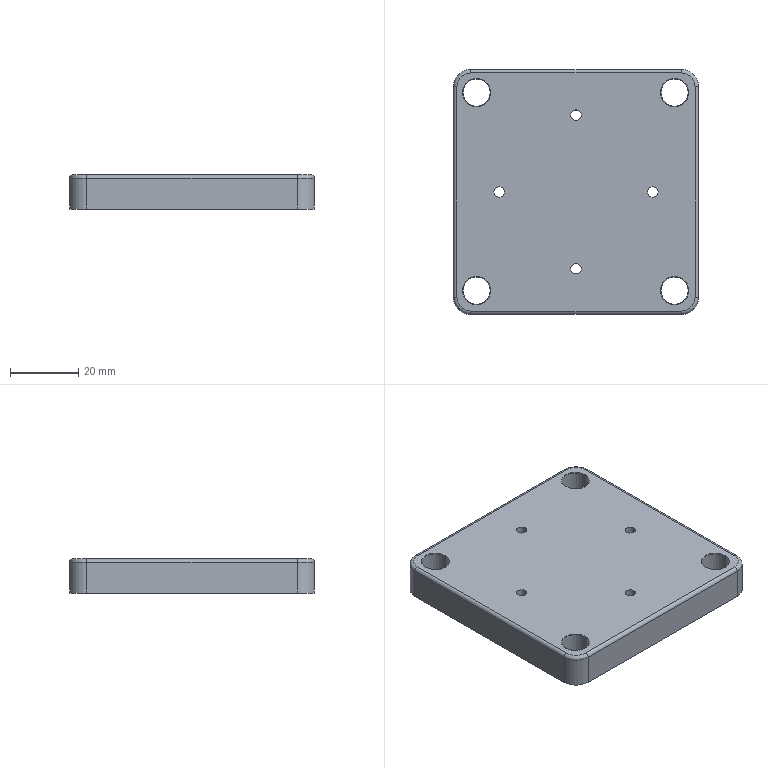Part | SolidWorks | features Fillet 3, Extrusion 1, ICE 1 | 1 solid | 42 faces | box 71.75 x 71.75 x 10 mm | volume 48903 mm3 | cylinder 24 | torus 12 | plane 6 | commonest cylinder face diameters 3.05 x8 8 x8 2 x4 10 x4
STEP:
#1=CARTESIAN_POINT('',(-1.525,22.5,0.));
#2=VERTEX_POINT('',#1);
#3=CARTESIAN_POINT('',(1.525,22.5,0.));
#4=VERTEX_POINT('',#3);
#5=CARTESIAN_POINT('',(0.,22.5,0.));
#6=DIRECTION('',(0.,0.,1.));
#7=DIRECTION('',(1.,0.,0.));
#8=AXIS2_PLACEMENT_3D('',#5,#6,#7);
#9=CIRCLE('',#8,1.525);
#10=EDGE_CURVE('',#2,#4,#9,.T.);
#11=ORIENTED_EDGE('',*,*,#10,.F.);
#12=CARTESIAN_POINT('',(-1.525,22.5,10.));
#13=VERTEX_POINT('',#12);
#14=CARTESIAN_POINT('',(-1.525,22.5,0.));
#15=DIRECTION('',(0.,0.,1.));
#16=VECTOR('',#15,1000.);
#17=LINE('',#14,#16);
#18=EDGE_CURVE('',#2,#13,#17,.T.);
#19=ORIENTED_EDGE('',*,*,#18,.T.);
#20=CARTESIAN_POINT('',(1.525,22.5,10.));
#21=VERTEX_POINT('',#20);
#22=CARTESIAN_POINT('',(0.,22.5,10.));
#23=DIRECTION('',(0.,0.,1.));
#24=DIRECTION('',(1.,0.,0.));
#25=AXIS2_PLACEMENT_3D('',#22,#23,#24);
#26=CIRCLE('',#25,1.525);
#27=EDGE_CURVE('',#13,#21,#26,.T.);
#28=ORIENTED_EDGE('',*,*,#27,.T.);
#29=CARTESIAN_POINT('',(1.525,22.5,0.));
#30=DIRECTION('',(0.,0.,1.));
#31=VECTOR('',#30,1000.);
#32=LINE('',#29,#31);
#33=EDGE_CURVE('',#4,#21,#32,.T.);
#34=ORIENTED_EDGE('',*,*,#33,.F.);
#35=EDGE_LOOP('',(#11,#19,#28,#34));
#36=FACE_OUTER_BOUND('',#35,.T.);
#37=CARTESIAN_POINT('',(0.,22.5,0.));
#38=DIRECTION('',(0.,0.,1.));
#39=DIRECTION('',(1.,0.,0.));
#40=AXIS2_PLACEMENT_3D('',#37,#38,#39);
#41=CYLINDRICAL_SURFACE('',#40,1.525);
#42=ADVANCED_FACE('',(#36),#41,.F.);
#43=CARTESIAN_POINT('',(20.975,0.,0.));
#44=VERTEX_POINT('',#43);
#45=CARTESIAN_POINT('',(24.025,0.,0.));
#46=VERTEX_POINT('',#45);
#47=CARTESIAN_POINT('',(22.5,0.,0.));
#48=DIRECTION('',(0.,0.,1.));
#49=DIRECTION('',(1.,0.,0.));
#50=AXIS2_PLACEMENT_3D('',#47,#48,#49);
#51=CIRCLE('',#50,1.525);
#52=EDGE_CURVE('',#44,#46,#51,.T.);
#53=ORIENTED_EDGE('',*,*,#52,.F.);
#54=CARTESIAN_POINT('',(20.975,0.,10.));
#55=VERTEX_POINT('',#54);
#56=CARTESIAN_POINT('',(20.975,0.,0.));
#57=DIRECTION('',(0.,0.,1.));
#58=VECTOR('',#57,1000.);
#59=LINE('',#56,#58);
#60=EDGE_CURVE('',#44,#55,#59,.T.);
#61=ORIENTED_EDGE('',*,*,#60,.T.);
#62=CARTESIAN_POINT('',(24.025,0.,10.));
#63=VERTEX_POINT('',#62);
#64=CARTESIAN_POINT('',(22.5,0.,10.));
#65=DIRECTION('',(0.,0.,1.));
#66=DIRECTION('',(1.,0.,0.));
#67=AXIS2_PLACEMENT_3D('',#64,#65,#66);
#68=CIRCLE('',#67,1.525);
#69=EDGE_CURVE('',#55,#63,#68,.T.);
#70=ORIENTED_EDGE('',*,*,#69,.T.);
#71=CARTESIAN_POINT('',(24.025,0.,0.));
#72=DIRECTION('',(0.,0.,1.));
#73=VECTOR('',#72,1000.);
#74=LINE('',#71,#73);
#75=EDGE_CURVE('',#46,#63,#74,.T.);
#76=ORIENTED_EDGE('',*,*,#75,.F.);
#77=EDGE_LOOP('',(#53,#61,#70,#76));
#78=FACE_OUTER_BOUND('',#77,.T.);
#79=CARTESIAN_POINT('',(22.5,0.,0.));
#80=DIRECTION('',(0.,0.,1.));
#81=DIRECTION('',(1.,0.,0.));
#82=AXIS2_PLACEMENT_3D('',#79,#80,#81);
#83=CYLINDRICAL_SURFACE('',#82,1.525);
#84=ADVANCED_FACE('',(#78),#83,.F.);
#85=CARTESIAN_POINT('',(-1.525,-22.5,0.));
#86=VERTEX_POINT('',#85);
#87=CARTESIAN_POINT('',(1.525,-22.5,0.));
#88=VERTEX_POINT('',#87);
#89=CARTESIAN_POINT('',(0.,-22.5,0.));
#90=DIRECTION('',(0.,0.,1.));
#91=DIRECTION('',(1.,0.,0.));
#92=AXIS2_PLACEMENT_3D('',#89,#90,#91);
#93=CIRCLE('',#92,1.525);
#94=EDGE_CURVE('',#86,#88,#93,.T.);
#95=ORIENTED_EDGE('',*,*,#94,.F.);
#96=CARTESIAN_POINT('',(-1.525,-22.5,10.));
#97=VERTEX_POINT('',#96);
#98=CARTESIAN_POINT('',(-1.525,-22.5,0.));
#99=DIRECTION('',(0.,0.,1.));
#100=VECTOR('',#99,1000.);
#101=LINE('',#98,#100);
#102=EDGE_CURVE('',#86,#97,#101,.T.);
#103=ORIENTED_EDGE('',*,*,#102,.T.);
#104=CARTESIAN_POINT('',(1.525,-22.5,10.));
#105=VERTEX_POINT('',#104);
#106=CARTESIAN_POINT('',(0.,-22.5,10.));
#107=DIRECTION('',(0.,0.,1.));
#108=DIRECTION('',(1.,0.,0.));
#109=AXIS2_PLACEMENT_3D('',#106,#107,#108);
#110=CIRCLE('',#109,1.525);
#111=EDGE_CURVE('',#97,#105,#110,.T.);
#112=ORIENTED_EDGE('',*,*,#111,.T.);
#113=CARTESIAN_POINT('',(1.525,-22.5,0.));
#114=DIRECTION('',(0.,0.,1.));
#115=VECTOR('',#114,1000.);
#116=LINE('',#113,#115);
#117=EDGE_CURVE('',#88,#105,#116,.T.);
#118=ORIENTED_EDGE('',*,*,#117,.F.);
#119=EDGE_LOOP('',(#95,#103,#112,#118));
#120=FACE_OUTER_BOUND('',#119,.T.);
#121=CARTESIAN_POINT('',(0.,-22.5,0.));
#122=DIRECTION('',(0.,0.,1.));
#123=DIRECTION('',(1.,0.,0.));
#124=AXIS2_PLACEMENT_3D('',#121,#122,#123);
#125=CYLINDRICAL_SURFACE('',#124,1.525);
#126=ADVANCED_FACE('',(#120),#125,.F.);
#127=CARTESIAN_POINT('',(-24.025,0.,0.));
#128=VERTEX_POINT('',#127);
#129=CARTESIAN_POINT('',(-20.975,0.,0.));
#130=VERTEX_POINT('',#129);
#131=CARTESIAN_POINT('',(-22.5,0.,0.));
#132=DIRECTION('',(0.,0.,1.));
#133=DIRECTION('',(1.,0.,0.));
#134=AXIS2_PLACEMENT_3D('',#131,#132,#133);
#135=CIRCLE('',#134,1.525);
#136=EDGE_CURVE('',#128,#130,#135,.T.);
#137=ORIENTED_EDGE('',*,*,#136,.F.);
#138=CARTESIAN_POINT('',(-24.025,0.,10.));
#139=VERTEX_POINT('',#138);
#140=CARTESIAN_POINT('',(-24.025,0.,0.));
#141=DIRECTION('',(0.,0.,1.));
#142=VECTOR('',#141,1000.);
#143=LINE('',#140,#142);
#144=EDGE_CURVE('',#128,#139,#143,.T.);
#145=ORIENTED_EDGE('',*,*,#144,.T.);
#146=CARTESIAN_POINT('',(-20.975,0.,10.));
#147=VERTEX_POINT('',#146);
#148=CARTESIAN_POINT('',(-22.5,0.,10.));
#149=DIRECTION('',(0.,0.,1.));
#150=DIRECTION('',(1.,0.,0.));
#151=AXIS2_PLACEMENT_3D('',#148,#149,#150);
#152=CIRCLE('',#151,1.525);
#153=EDGE_CURVE('',#139,#147,#152,.T.);
#154=ORIENTED_EDGE('',*,*,#153,.T.);
#155=CARTESIAN_POINT('',(-20.975,0.,0.));
#156=DIRECTION('',(0.,0.,1.));
#157=VECTOR('',#156,1000.);
#158=LINE('',#155,#157);
#159=EDGE_CURVE('',#130,#147,#158,.T.);
#160=ORIENTED_EDGE('',*,*,#159,.F.);
#161=EDGE_LOOP('',(#137,#145,#154,#160));
#162=FACE_OUTER_BOUND('',#161,.T.);
#163=CARTESIAN_POINT('',(-22.5,0.,0.));
#164=DIRECTION('',(0.,0.,1.));
#165=DIRECTION('',(1.,0.,0.));
#166=AXIS2_PLACEMENT_3D('',#163,#164,#165);
#167=CYLINDRICAL_SURFACE('',#166,1.525);
#168=ADVANCED_FACE('',(#162),#167,.F.);
#169=CARTESIAN_POINT('',(24.725,29.125,10.));
#170=VERTEX_POINT('',#169);
#171=CARTESIAN_POINT('',(33.025,29.125,10.));
#172=VERTEX_POINT('',#171);
#173=CARTESIAN_POINT('',(28.875,29.125,10.));
#174=DIRECTION('',(0.,0.,-1.));
#175=DIRECTION('',(1.,0.,0.));
#176=AXIS2_PLACEMENT_3D('',#173,#174,#175);
#177=CIRCLE('',#176,4.15);
#178=EDGE_CURVE('',#170,#172,#177,.T.);
#179=ORIENTED_EDGE('',*,*,#178,.F.);
#180=CARTESIAN_POINT('',(24.875,29.125,9.85));
#181=VERTEX_POINT('',#180);
#182=CARTESIAN_POINT('',(24.725,29.125,9.85));
#183=DIRECTION('',(0.,1.,0.));
#184=DIRECTION('',(-1.,0.,0.));
#185=AXIS2_PLACEMENT_3D('',#182,#183,#184);
#186=CIRCLE('',#185,0.15);
#187=EDGE_CURVE('',#170,#181,#186,.T.);
#188=ORIENTED_EDGE('',*,*,#187,.T.);
#189=CARTESIAN_POINT('',(32.875,29.125,9.85));
#190=VERTEX_POINT('',#189);
#191=CARTESIAN_POINT('',(28.875,29.125,9.85));
#192=DIRECTION('',(0.,0.,1.));
#193=DIRECTION('',(1.,0.,0.));
#194=AXIS2_PLACEMENT_3D('',#191,#192,#193);
#195=CIRCLE('',#194,4.);
#196=EDGE_CURVE('',#190,#181,#195,.T.);
#197=ORIENTED_EDGE('',*,*,#196,.F.);
#198=CARTESIAN_POINT('',(33.025,29.125,9.85));
#199=DIRECTION('',(0.,-1.,0.));
#200=DIRECTION('',(0.,0.,-1.));
#201=AXIS2_PLACEMENT_3D('',#198,#199,#200);
#202=CIRCLE('',#201,0.15);
#203=EDGE_CURVE('',#172,#190,#202,.T.);
#204=ORIENTED_EDGE('',*,*,#203,.F.);
#205=EDGE_LOOP('',(#179,#188,#197,#204));
#206=FACE_OUTER_BOUND('',#205,.T.);
#207=CARTESIAN_POINT('',(28.875,29.125,9.85));
#208=DIRECTION('',(0.,0.,1.));
#209=DIRECTION('',(1.,0.,0.));
#210=AXIS2_PLACEMENT_3D('',#207,#208,#209);
#211=TOROIDAL_SURFACE('',#210,4.15,0.15);
#212=ADVANCED_FACE('',(#206),#211,.T.);
#213=CARTESIAN_POINT('',(-33.275,29.125,10.));
#214=VERTEX_POINT('',#213);
#215=CARTESIAN_POINT('',(-24.975,29.125,10.));
#216=VERTEX_POINT('',#215);
#217=CARTESIAN_POINT('',(-29.125,29.125,10.));
#218=DIRECTION('',(0.,0.,-1.));
#219=DIRECTION('',(1.,0.,0.));
#220=AXIS2_PLACEMENT_3D('',#217,#218,#219);
#221=CIRCLE('',#220,4.15);
#222=EDGE_CURVE('',#214,#216,#221,.T.);
#223=ORIENTED_EDGE('',*,*,#222,.F.);
#224=CARTESIAN_POINT('',(-33.125,29.125,9.85));
#225=VERTEX_POINT('',#224);
#226=CARTESIAN_POINT('',(-33.275,29.125,9.85));
#227=DIRECTION('',(0.,1.,0.));
#228=DIRECTION('',(-1.,0.,0.));
#229=AXIS2_PLACEMENT_3D('',#226,#227,#228);
#230=CIRCLE('',#229,0.15);
#231=EDGE_CURVE('',#214,#225,#230,.T.);
#232=ORIENTED_EDGE('',*,*,#231,.T.);
#233=CARTESIAN_POINT('',(-25.125,29.125,9.85));
#234=VERTEX_POINT('',#233);
#235=CARTESIAN_POINT('',(-29.125,29.125,9.85));
#236=DIRECTION('',(0.,0.,1.));
#237=DIRECTION('',(1.,0.,0.));
#238=AXIS2_PLACEMENT_3D('',#235,#236,#237);
#239=CIRCLE('',#238,4.);
#240=EDGE_CURVE('',#234,#225,#239,.T.);
#241=ORIENTED_EDGE('',*,*,#240,.F.);
#242=CARTESIAN_POINT('',(-24.975,29.125,9.85));
#243=DIRECTION('',(0.,-1.,0.));
#244=DIRECTION('',(0.,0.,-1.));
#245=AXIS2_PLACEMENT_3D('',#242,#243,#244);
#246=CIRCLE('',#245,0.15);
#247=EDGE_CURVE('',#216,#234,#246,.T.);
#248=ORIENTED_EDGE('',*,*,#247,.F.);
#249=EDGE_LOOP('',(#223,#232,#241,#248));
#250=FACE_OUTER_BOUND('',#249,.T.);
#251=CARTESIAN_POINT('',(-29.125,29.125,9.85));
#252=DIRECTION('',(0.,0.,1.));
#253=DIRECTION('',(1.,0.,0.));
#254=AXIS2_PLACEMENT_3D('',#251,#252,#253);
#255=TOROIDAL_SURFACE('',#254,4.15,0.15);
#256=ADVANCED_FACE('',(#250),#255,.T.);
#257=CARTESIAN_POINT('',(-33.275,-28.875,10.));
#258=VERTEX_POINT('',#257);
#259=CARTESIAN_POINT('',(-24.975,-28.875,10.));
#260=VERTEX_POINT('',#259);
#261=CARTESIAN_POINT('',(-29.125,-28.875,10.));
#262=DIRECTION('',(0.,0.,-1.));
#263=DIRECTION('',(1.,0.,0.));
#264=AXIS2_PLACEMENT_3D('',#261,#262,#263);
#265=CIRCLE('',#264,4.15);
#266=EDGE_CURVE('',#258,#260,#265,.T.);
#267=ORIENTED_EDGE('',*,*,#266,.F.);
#268=CARTESIAN_POINT('',(-33.125,-28.875,9.85));
#269=VERTEX_POINT('',#268);
#270=CARTESIAN_POINT('',(-33.275,-28.875,9.85));
#271=DIRECTION('',(0.,1.,0.));
#272=DIRECTION('',(-1.,0.,0.));
#273=AXIS2_PLACEMENT_3D('',#270,#271,#272);
#274=CIRCLE('',#273,0.15);
#275=EDGE_CURVE('',#258,#269,#274,.T.);
#276=ORIENTED_EDGE('',*,*,#275,.T.);
#277=CARTESIAN_POINT('',(-25.125,-28.875,9.85));
#278=VERTEX_POINT('',#277);
#279=CARTESIAN_POINT('',(-29.125,-28.875,9.85));
#280=DIRECTION('',(0.,0.,1.));
#281=DIRECTION('',(1.,0.,0.));
#282=AXIS2_PLACEMENT_3D('',#279,#280,#281);
#283=CIRCLE('',#282,4.);
#284=EDGE_CURVE('',#278,#269,#283,.T.);
#285=ORIENTED_EDGE('',*,*,#284,.F.);
#286=CARTESIAN_POINT('',(-24.975,-28.875,9.85));
#287=DIRECTION('',(0.,-1.,0.));
#288=DIRECTION('',(0.,0.,-1.));
#289=AXIS2_PLACEMENT_3D('',#286,#287,#288);
#290=CIRCLE('',#289,0.15);
#291=EDGE_CURVE('',#260,#278,#290,.T.);
#292=ORIENTED_EDGE('',*,*,#291,.F.);
#293=EDGE_LOOP('',(#267,#276,#285,#292));
#294=FACE_OUTER_BOUND('',#293,.T.);
#295=CARTESIAN_POINT('',(-29.125,-28.875,9.85));
#296=DIRECTION('',(0.,0.,1.));
#297=DIRECTION('',(1.,0.,0.));
#298=AXIS2_PLACEMENT_3D('',#295,#296,#297);
#299=TOROIDAL_SURFACE('',#298,4.15,0.15);
#300=ADVANCED_FACE('',(#294),#299,.T.);
#301=CARTESIAN_POINT('',(24.725,-28.875,10.));
#302=VERTEX_POINT('',#301);
#303=CARTESIAN_POINT('',(33.025,-28.875,10.));
#304=VERTEX_POINT('',#303);
#305=CARTESIAN_POINT('',(28.875,-28.875,10.));
#306=DIRECTION('',(0.,0.,-1.));
#307=DIRECTION('',(1.,0.,0.));
#308=AXIS2_PLACEMENT_3D('',#305,#306,#307);
#309=CIRCLE('',#308,4.15);
#310=EDGE_CURVE('',#302,#304,#309,.T.);
#311=ORIENTED_EDGE('',*,*,#310,.F.);
#312=CARTESIAN_POINT('',(24.875,-28.875,9.85));
#313=VERTEX_POINT('',#312);
#314=CARTESIAN_POINT('',(24.725,-28.875,9.85));
#315=DIRECTION('',(0.,1.,0.));
#316=DIRECTION('',(-1.,0.,0.));
#317=AXIS2_PLACEMENT_3D('',#314,#315,#316);
#318=CIRCLE('',#317,0.15);
#319=EDGE_CURVE('',#302,#313,#318,.T.);
#320=ORIENTED_EDGE('',*,*,#319,.T.);
#321=CARTESIAN_POINT('',(32.875,-28.875,9.85));
#322=VERTEX_POINT('',#321);
#323=CARTESIAN_POINT('',(28.875,-28.875,9.85));
#324=DIRECTION('',(0.,0.,1.));
#325=DIRECTION('',(1.,0.,0.));
#326=AXIS2_PLACEMENT_3D('',#323,#324,#325);
#327=CIRCLE('',#326,4.);
#328=EDGE_CURVE('',#322,#313,#327,.T.);
#329=ORIENTED_EDGE('',*,*,#328,.F.);
#330=CARTESIAN_POINT('',(33.025,-28.875,9.85));
#331=DIRECTION('',(0.,-1.,0.));
#332=DIRECTION('',(0.,0.,-1.));
#333=AXIS2_PLACEMENT_3D('',#330,#331,#332);
#334=CIRCLE('',#333,0.15);
#335=EDGE_CURVE('',#304,#322,#334,.T.);
#336=ORIENTED_EDGE('',*,*,#335,.F.);
#337=EDGE_LOOP('',(#311,#320,#329,#336));
#338=FACE_OUTER_BOUND('',#337,.T.);
#339=CARTESIAN_POINT('',(28.875,-28.875,9.85));
#340=DIRECTION('',(0.,0.,1.));
#341=DIRECTION('',(1.,0.,0.));
#342=AXIS2_PLACEMENT_3D('',#339,#340,#341);
#343=TOROIDAL_SURFACE('',#342,4.15,0.15);
#344=ADVANCED_FACE('',(#338),#343,.T.);
#345=CARTESIAN_POINT('',(-29.125,-28.875,9.85));
#346=DIRECTION('',(0.,0.,1.));
#347=DIRECTION('',(1.,0.,0.));
#348=AXIS2_PLACEMENT_3D('',#345,#346,#347);
#349=CIRCLE('',#348,4.);
#350=EDGE_CURVE('',#269,#278,#349,.T.);
#351=ORIENTED_EDGE('',*,*,#350,.T.);
#352=CARTESIAN_POINT('',(-25.125,-28.875,0.));
#353=VERTEX_POINT('',#352);
#354=CARTESIAN_POINT('',(-25.125,-28.875,10.));
#355=DIRECTION('',(0.,0.,-1.));
#356=VECTOR('',#355,1000.);
#357=LINE('',#354,#356);
#358=EDGE_CURVE('',#278,#353,#357,.T.);
#359=ORIENTED_EDGE('',*,*,#358,.T.);
#360=CARTESIAN_POINT('',(-33.125,-28.875,0.));
#361=VERTEX_POINT('',#360);
#362=CARTESIAN_POINT('',(-29.125,-28.875,0.));
#363=DIRECTION('',(0.,0.,1.));
#364=DIRECTION('',(1.,0.,0.));
#365=AXIS2_PLACEMENT_3D('',#362,#363,#364);
#366=CIRCLE('',#365,4.);
#367=EDGE_CURVE('',#361,#353,#366,.T.);
#368=ORIENTED_EDGE('',*,*,#367,.F.);
#369=CARTESIAN_POINT('',(-33.125,-28.875,10.));
#370=DIRECTION('',(0.,0.,-1.));
#371=VECTOR('',#370,1000.);
#372=LINE('',#369,#371);
#373=EDGE_CURVE('',#269,#361,#372,.T.);
#374=ORIENTED_EDGE('',*,*,#373,.F.);
#375=EDGE_LOOP('',(#351,#359,#368,#374));
#376=FACE_OUTER_BOUND('',#375,.T.);
#377=CARTESIAN_POINT('',(-29.125,-28.875,10.));
#378=DIRECTION('',(0.,0.,-1.));
#379=DIRECTION('',(-1.,0.,0.));
#380=AXIS2_PLACEMENT_3D('',#377,#378,#379);
#381=CYLINDRICAL_SURFACE('',#380,4.);
#382=ADVANCED_FACE('',(#376),#381,.F.);
#383=CARTESIAN_POINT('',(28.875,-28.875,9.85));
#384=DIRECTION('',(0.,0.,1.));
#385=DIRECTION('',(1.,0.,0.));
#386=AXIS2_PLACEMENT_3D('',#383,#384,#385);
#387=CIRCLE('',#386,4.);
#388=EDGE_CURVE('',#313,#322,#387,.T.);
#389=ORIENTED_EDGE('',*,*,#388,.T.);
#390=CARTESIAN_POINT('',(32.875,-28.875,0.));
#391=VERTEX_POINT('',#390);
#392=CARTESIAN_POINT('',(32.875,-28.875,10.));
#393=DIRECTION('',(0.,0.,-1.));
#394=VECTOR('',#393,1000.);
#395=LINE('',#392,#394);
#396=EDGE_CURVE('',#322,#391,#395,.T.);
#397=ORIENTED_EDGE('',*,*,#396,.T.);
#398=CARTESIAN_POINT('',(24.875,-28.875,0.));
#399=VERTEX_POINT('',#398);
#400=CARTESIAN_POINT('',(28.875,-28.875,0.));
#401=DIRECTION('',(0.,0.,1.));
#402=DIRECTION('',(1.,0.,0.));
#403=AXIS2_PLACEMENT_3D('',#400,#401,#402);
#404=CIRCLE('',#403,4.);
#405=EDGE_CURVE('',#399,#391,#404,.T.);
#406=ORIENTED_EDGE('',*,*,#405,.F.);
#407=CARTESIAN_POINT('',(24.875,-28.875,10.));
#408=DIRECTION('',(0.,0.,-1.));
#409=VECTOR('',#408,1000.);
#410=LINE('',#407,#409);
#411=EDGE_CURVE('',#313,#399,#410,.T.);
#412=ORIENTED_EDGE('',*,*,#411,.F.);
#413=EDGE_LOOP('',(#389,#397,#406,#412));
#414=FACE_OUTER_BOUND('',#413,.T.);
#415=CARTESIAN_POINT('',(28.875,-28.875,10.));
#416=DIRECTION('',(0.,0.,-1.));
#417=DIRECTION('',(-1.,0.,0.));
#418=AXIS2_PLACEMENT_3D('',#415,#416,#417);
#419=CYLINDRICAL_SURFACE('',#418,4.);
#420=ADVANCED_FACE('',(#414),#419,.F.);
#421=CARTESIAN_POINT('',(28.875,29.125,9.85));
#422=DIRECTION('',(0.,0.,1.));
#423=DIRECTION('',(1.,0.,0.));
#424=AXIS2_PLACEMENT_3D('',#421,#422,#423);
#425=CIRCLE('',#424,4.);
#426=EDGE_CURVE('',#181,#190,#425,.T.);
#427=ORIENTED_EDGE('',*,*,#426,.T.);
#428=CARTESIAN_POINT('',(32.875,29.125,0.));
#429=VERTEX_POINT('',#428);
#430=CARTESIAN_POINT('',(32.875,29.125,10.));
#431=DIRECTION('',(0.,0.,-1.));
#432=VECTOR('',#431,1000.);
#433=LINE('',#430,#432);
#434=EDGE_CURVE('',#190,#429,#433,.T.);
#435=ORIENTED_EDGE('',*,*,#434,.T.);
#436=CARTESIAN_POINT('',(24.875,29.125,0.));
#437=VERTEX_POINT('',#436);
#438=CARTESIAN_POINT('',(28.875,29.125,0.));
#439=DIRECTION('',(0.,0.,1.));
#440=DIRECTION('',(1.,0.,0.));
#441=AXIS2_PLACEMENT_3D('',#438,#439,#440);
#442=CIRCLE('',#441,4.);
#443=EDGE_CURVE('',#437,#429,#442,.T.);
#444=ORIENTED_EDGE('',*,*,#443,.F.);
#445=CARTESIAN_POINT('',(24.875,29.125,10.));
#446=DIRECTION('',(0.,0.,-1.));
#447=VECTOR('',#446,1000.);
#448=LINE('',#445,#447);
#449=EDGE_CURVE('',#181,#437,#448,.T.);
#450=ORIENTED_EDGE('',*,*,#449,.F.);
#451=EDGE_LOOP('',(#427,#435,#444,#450));
#452=FACE_OUTER_BOUND('',#451,.T.);
#453=CARTESIAN_POINT('',(28.875,29.125,10.));
#454=DIRECTION('',(0.,0.,-1.));
#455=DIRECTION('',(-1.,0.,0.));
#456=AXIS2_PLACEMENT_3D('',#453,#454,#455);
#457=CYLINDRICAL_SURFACE('',#456,4.);
#458=ADVANCED_FACE('',(#452),#457,.F.);
#459=CARTESIAN_POINT('',(-29.125,29.125,9.85));
#460=DIRECTION('',(0.,0.,1.));
#461=DIRECTION('',(1.,0.,0.));
#462=AXIS2_PLACEMENT_3D('',#459,#460,#461);
#463=CIRCLE('',#462,4.);
#464=EDGE_CURVE('',#225,#234,#463,.T.);
#465=ORIENTED_EDGE('',*,*,#464,.T.);
#466=CARTESIAN_POINT('',(-25.125,29.125,0.));
#467=VERTEX_POINT('',#466);
#468=CARTESIAN_POINT('',(-25.125,29.125,10.));
#469=DIRECTION('',(0.,0.,-1.));
#470=VECTOR('',#469,1000.);
#471=LINE('',#468,#470);
#472=EDGE_CURVE('',#234,#467,#471,.T.);
#473=ORIENTED_EDGE('',*,*,#472,.T.);
#474=CARTESIAN_POINT('',(-33.125,29.125,0.));
#475=VERTEX_POINT('',#474);
#476=CARTESIAN_POINT('',(-29.125,29.125,0.));
#477=DIRECTION('',(0.,0.,1.));
#478=DIRECTION('',(1.,0.,0.));
#479=AXIS2_PLACEMENT_3D('',#476,#477,#478);
#480=CIRCLE('',#479,4.);
#481=EDGE_CURVE('',#475,#467,#480,.T.);
#482=ORIENTED_EDGE('',*,*,#481,.F.);
#483=CARTESIAN_POINT('',(-33.125,29.125,10.));
#484=DIRECTION('',(0.,0.,-1.));
#485=VECTOR('',#484,1000.);
#486=LINE('',#483,#485);
#487=EDGE_CURVE('',#225,#475,#486,.T.);
#488=ORIENTED_EDGE('',*,*,#487,.F.);
#489=EDGE_LOOP('',(#465,#473,#482,#488));
#490=FACE_OUTER_BOUND('',#489,.T.);
#491=CARTESIAN_POINT('',(-29.125,29.125,10.));
#492=DIRECTION('',(0.,0.,-1.));
#493=DIRECTION('',(-1.,0.,0.));
#494=AXIS2_PLACEMENT_3D('',#491,#492,#493);
#495=CYLINDRICAL_SURFACE('',#494,4.);
#496=ADVANCED_FACE('',(#490),#495,.F.);
#497=CARTESIAN_POINT('',(0.,22.5,10.));
#498=DIRECTION('',(0.,0.,1.));
#499=DIRECTION('',(1.,0.,0.));
#500=AXIS2_PLACEMENT_3D('',#497,#498,#499);
#501=CIRCLE('',#500,1.525);
#502=EDGE_CURVE('',#21,#13,#501,.T.);
#503=ORIENTED_EDGE('',*,*,#502,.F.);
#504=ORIENTED_EDGE('',*,*,#27,.F.);
#505=EDGE_LOOP('',(#503,#504));
#506=FACE_BOUND('',#505,.T.);
#507=CARTESIAN_POINT('',(22.5,0.,10.));
#508=DIRECTION('',(0.,0.,1.));
#509=DIRECTION('',(1.,0.,0.));
#510=AXIS2_PLACEMENT_3D('',#507,#508,#509);
#511=CIRCLE('',#510,1.525);
#512=EDGE_CURVE('',#63,#55,#511,.T.);
#513=ORIENTED_EDGE('',*,*,#512,.F.);
#514=ORIENTED_EDGE('',*,*,#69,.F.);
#515=EDGE_LOOP('',(#513,#514));
#516=FACE_BOUND('',#515,.T.);
#517=CARTESIAN_POINT('',(0.,-22.5,10.));
#518=DIRECTION('',(0.,0.,1.));
#519=DIRECTION('',(1.,0.,0.));
#520=AXIS2_PLACEMENT_3D('',#517,#518,#519);
#521=CIRCLE('',#520,1.525);
#522=EDGE_CURVE('',#105,#97,#521,.T.);
#523=ORIENTED_EDGE('',*,*,#522,.F.);
#524=ORIENTED_EDGE('',*,*,#111,.F.);
#525=EDGE_LOOP('',(#523,#524));
#526=FACE_BOUND('',#525,.T.);
#527=CARTESIAN_POINT('',(-22.5,0.,10.));
#528=DIRECTION('',(0.,0.,1.));
#529=DIRECTION('',(1.,0.,0.));
#530=AXIS2_PLACEMENT_3D('',#527,#528,#529);
#531=CIRCLE('',#530,1.525);
#532=EDGE_CURVE('',#147,#139,#531,.T.);
#533=ORIENTED_EDGE('',*,*,#532,.F.);
#534=ORIENTED_EDGE('',*,*,#153,.F.);
#535=EDGE_LOOP('',(#533,#534));
#536=FACE_BOUND('',#535,.T.);
#537=CARTESIAN_POINT('',(28.875,-28.875,10.));
#538=DIRECTION('',(0.,0.,-1.));
#539=DIRECTION('',(1.,0.,0.));
#540=AXIS2_PLACEMENT_3D('',#537,#538,#539);
#541=CIRCLE('',#540,4.15);
#542=EDGE_CURVE('',#304,#302,#541,.T.);
#543=ORIENTED_EDGE('',*,*,#542,.T.);
#544=ORIENTED_EDGE('',*,*,#310,.T.);
#545=EDGE_LOOP('',(#543,#544));
#546=FACE_BOUND('',#545,.T.);
#547=CARTESIAN_POINT('',(-29.125,-28.875,10.));
#548=DIRECTION('',(0.,0.,-1.));
#549=DIRECTION('',(1.,0.,0.));
#550=AXIS2_PLACEMENT_3D('',#547,#548,#549);
#551=CIRCLE('',#550,4.15);
#552=EDGE_CURVE('',#260,#258,#551,.T.);
#553=ORIENTED_EDGE('',*,*,#552,.T.);
#554=ORIENTED_EDGE('',*,*,#266,.T.);
#555=EDGE_LOOP('',(#553,#554));
#556=FACE_BOUND('',#555,.T.);
#557=CARTESIAN_POINT('',(-29.125,29.125,10.));
#558=DIRECTION('',(0.,0.,-1.));
#559=DIRECTION('',(1.,0.,0.));
#560=AXIS2_PLACEMENT_3D('',#557,#558,#559);
#561=CIRCLE('',#560,4.15);
#562=EDGE_CURVE('',#216,#214,#561,.T.);
#563=ORIENTED_EDGE('',*,*,#562,.T.);
#564=ORIENTED_EDGE('',*,*,#222,.T.);
#565=EDGE_LOOP('',(#563,#564));
#566=FACE_BOUND('',#565,.T.);
#567=CARTESIAN_POINT('',(28.875,29.125,10.));
#568=DIRECTION('',(0.,0.,-1.));
#569=DIRECTION('',(1.,0.,0.));
#570=AXIS2_PLACEMENT_3D('',#567,#568,#569);
#571=CIRCLE('',#570,4.15);
#572=EDGE_CURVE('',#172,#170,#571,.T.);
#573=ORIENTED_EDGE('',*,*,#572,.T.);
#574=ORIENTED_EDGE('',*,*,#178,.T.);
#575=EDGE_LOOP('',(#573,#574));
#576=FACE_BOUND('',#575,.T.);
#577=CARTESIAN_POINT('',(-34.875,-30.875,10.));
#578=VERTEX_POINT('',#577);
#579=CARTESIAN_POINT('',(-30.875,-34.875,10.));
#580=VERTEX_POINT('',#579);
#581=CARTESIAN_POINT('',(-30.875,-30.875,10.));
#582=DIRECTION('',(0.,0.,1.));
#583=DIRECTION('',(1.,0.,0.));
#584=AXIS2_PLACEMENT_3D('',#581,#582,#583);
#585=CIRCLE('',#584,4.);
#586=EDGE_CURVE('',#578,#580,#585,.T.);
#587=ORIENTED_EDGE('',*,*,#586,.T.);
#588=CARTESIAN_POINT('',(30.875,-34.875,10.));
#589=VERTEX_POINT('',#588);
#590=CARTESIAN_POINT('',(30.875,-34.875,10.));
#591=DIRECTION('',(1.,0.,0.));
#592=VECTOR('',#591,1000.);
#593=LINE('',#590,#592);
#594=EDGE_CURVE('',#580,#589,#593,.T.);
#595=ORIENTED_EDGE('',*,*,#594,.T.);
#596=CARTESIAN_POINT('',(34.875,-30.875,10.));
#597=VERTEX_POINT('',#596);
#598=CARTESIAN_POINT('',(30.875,-30.875,10.));
#599=DIRECTION('',(0.,0.,1.));
#600=DIRECTION('',(1.,0.,0.));
#601=AXIS2_PLACEMENT_3D('',#598,#599,#600);
#602=CIRCLE('',#601,4.);
#603=EDGE_CURVE('',#589,#597,#602,.T.);
#604=ORIENTED_EDGE('',*,*,#603,.T.);
#605=CARTESIAN_POINT('',(34.875,30.875,10.));
#606=VERTEX_POINT('',#605);
#607=CARTESIAN_POINT('',(34.875,30.875,10.));
#608=DIRECTION('',(0.,1.,0.));
#609=VECTOR('',#608,1000.);
#610=LINE('',#607,#609);
#611=EDGE_CURVE('',#597,#606,#610,.T.);
#612=ORIENTED_EDGE('',*,*,#611,.T.);
#613=CARTESIAN_POINT('',(30.875,34.875,10.));
#614=VERTEX_POINT('',#613);
#615=CARTESIAN_POINT('',(30.875,30.875,10.));
#616=DIRECTION('',(0.,0.,1.));
#617=DIRECTION('',(1.,0.,0.));
#618=AXIS2_PLACEMENT_3D('',#615,#616,#617);
#619=CIRCLE('',#618,4.);
#620=EDGE_CURVE('',#606,#614,#619,.T.);
#621=ORIENTED_EDGE('',*,*,#620,.T.);
#622=CARTESIAN_POINT('',(-30.875,34.875,10.));
#623=VERTEX_POINT('',#622);
#624=CARTESIAN_POINT('',(-30.875,34.875,10.));
#625=DIRECTION('',(-1.,0.,0.));
#626=VECTOR('',#625,1000.);
#627=LINE('',#624,#626);
#628=EDGE_CURVE('',#614,#623,#627,.T.);
#629=ORIENTED_EDGE('',*,*,#628,.T.);
#630=CARTESIAN_POINT('',(-34.875,30.875,10.));
#631=VERTEX_POINT('',#630);
#632=CARTESIAN_POINT('',(-30.875,30.875,10.));
#633=DIRECTION('',(0.,0.,1.));
#634=DIRECTION('',(1.,0.,0.));
#635=AXIS2_PLACEMENT_3D('',#632,#633,#634);
#636=CIRCLE('',#635,4.);
#637=EDGE_CURVE('',#623,#631,#636,.T.);
#638=ORIENTED_EDGE('',*,*,#637,.T.);
#639=CARTESIAN_POINT('',(-34.875,-30.875,10.));
#640=DIRECTION('',(0.,-1.,0.));
#641=VECTOR('',#640,1000.);
#642=LINE('',#639,#641);
#643=EDGE_CURVE('',#631,#578,#642,.T.);
#644=ORIENTED_EDGE('',*,*,#643,.T.);
#645=EDGE_LOOP('',(#587,#595,#604,#612,#621,#629,#638,#644));
#646=FACE_OUTER_BOUND('',#645,.T.);
#647=CARTESIAN_POINT('',(0.,0.,10.));
#648=DIRECTION('',(0.,0.,1.));
#649=DIRECTION('',(1.,0.,0.));
#650=AXIS2_PLACEMENT_3D('',#647,#648,#649);
#651=PLANE('',#650);
#652=ADVANCED_FACE('',(#506,#516,#526,#536,#546,#556,#566,#576,#646),#651,.T.);
#653=CARTESIAN_POINT('',(0.,22.5,0.));
#654=DIRECTION('',(0.,0.,1.));
#655=DIRECTION('',(1.,0.,0.));
#656=AXIS2_PLACEMENT_3D('',#653,#654,#655);
#657=CIRCLE('',#656,1.525);
#658=EDGE_CURVE('',#4,#2,#657,.T.);
#659=ORIENTED_EDGE('',*,*,#658,.T.);
#660=ORIENTED_EDGE('',*,*,#10,.T.);
#661=EDGE_LOOP('',(#659,#660));
#662=FACE_BOUND('',#661,.T.);
#663=CARTESIAN_POINT('',(22.5,0.,0.));
#664=DIRECTION('',(0.,0.,1.));
#665=DIRECTION('',(1.,0.,0.));
#666=AXIS2_PLACEMENT_3D('',#663,#664,#665);
#667=CIRCLE('',#666,1.525);
#668=EDGE_CURVE('',#46,#44,#667,.T.);
#669=ORIENTED_EDGE('',*,*,#668,.T.);
#670=ORIENTED_EDGE('',*,*,#52,.T.);
#671=EDGE_LOOP('',(#669,#670));
#672=FACE_BOUND('',#671,.T.);
#673=CARTESIAN_POINT('',(0.,-22.5,0.));
#674=DIRECTION('',(0.,0.,1.));
#675=DIRECTION('',(1.,0.,0.));
#676=AXIS2_PLACEMENT_3D('',#673,#674,#675);
#677=CIRCLE('',#676,1.525);
#678=EDGE_CURVE('',#88,#86,#677,.T.);
#679=ORIENTED_EDGE('',*,*,#678,.T.);
#680=ORIENTED_EDGE('',*,*,#94,.T.);
#681=EDGE_LOOP('',(#679,#680));
#682=FACE_BOUND('',#681,.T.);
#683=CARTESIAN_POINT('',(-22.5,0.,0.));
#684=DIRECTION('',(0.,0.,1.));
#685=DIRECTION('',(1.,0.,0.));
#686=AXIS2_PLACEMENT_3D('',#683,#684,#685);
#687=CIRCLE('',#686,1.525);
#688=EDGE_CURVE('',#130,#128,#687,.T.);
#689=ORIENTED_EDGE('',*,*,#688,.T.);
#690=ORIENTED_EDGE('',*,*,#136,.T.);
#691=EDGE_LOOP('',(#689,#690));
#692=FACE_BOUND('',#691,.T.);
#693=CARTESIAN_POINT('',(35.875,-30.875,0.));
#694=VERTEX_POINT('',#693);
#695=CARTESIAN_POINT('',(35.875,30.875,0.));
#696=VERTEX_POINT('',#695);
#697=CARTESIAN_POINT('',(35.875,35.875,0.));
#698=DIRECTION('',(0.,1.,0.));
#699=VECTOR('',#698,1000.);
#700=LINE('',#697,#699);
#701=EDGE_CURVE('',#694,#696,#700,.T.);
#702=ORIENTED_EDGE('',*,*,#701,.F.);
#703=CARTESIAN_POINT('',(30.875,-35.875,0.));
#704=VERTEX_POINT('',#703);
#705=CARTESIAN_POINT('',(30.875,-30.875,0.));
#706=DIRECTION('',(0.,0.,-1.));
#707=DIRECTION('',(1.,0.,0.));
#708=AXIS2_PLACEMENT_3D('',#705,#706,#707);
#709=CIRCLE('',#708,5.);
#710=EDGE_CURVE('',#694,#704,#709,.T.);
#711=ORIENTED_EDGE('',*,*,#710,.T.);
#712=CARTESIAN_POINT('',(-30.875,-35.875,0.));
#713=VERTEX_POINT('',#712);
#714=CARTESIAN_POINT('',(-35.875,-35.875,0.));
#715=DIRECTION('',(1.,0.,0.));
#716=VECTOR('',#715,1000.);
#717=LINE('',#714,#716);
#718=EDGE_CURVE('',#713,#704,#717,.T.);
#719=ORIENTED_EDGE('',*,*,#718,.F.);
#720=CARTESIAN_POINT('',(-35.875,-30.875,0.));
#721=VERTEX_POINT('',#720);
#722=CARTESIAN_POINT('',(-30.875,-30.875,0.));
#723=DIRECTION('',(0.,0.,-1.));
#724=DIRECTION('',(1.,0.,0.));
#725=AXIS2_PLACEMENT_3D('',#722,#723,#724);
#726=CIRCLE('',#725,5.);
#727=EDGE_CURVE('',#713,#721,#726,.T.);
#728=ORIENTED_EDGE('',*,*,#727,.T.);
#729=CARTESIAN_POINT('',(-35.875,30.875,0.));
#730=VERTEX_POINT('',#729);
#731=CARTESIAN_POINT('',(-35.875,35.875,0.));
#732=DIRECTION('',(0.,-1.,0.));
#733=VECTOR('',#732,1000.);
#734=LINE('',#731,#733);
#735=EDGE_CURVE('',#730,#721,#734,.T.);
#736=ORIENTED_EDGE('',*,*,#735,.F.);
#737=CARTESIAN_POINT('',(-30.875,35.875,0.));
#738=VERTEX_POINT('',#737);
#739=CARTESIAN_POINT('',(-30.875,30.875,0.));
#740=DIRECTION('',(0.,0.,-1.));
#741=DIRECTION('',(1.,0.,0.));
#742=AXIS2_PLACEMENT_3D('',#739,#740,#741);
#743=CIRCLE('',#742,5.);
#744=EDGE_CURVE('',#730,#738,#743,.T.);
#745=ORIENTED_EDGE('',*,*,#744,.T.);
#746=CARTESIAN_POINT('',(30.875,35.875,0.));
#747=VERTEX_POINT('',#746);
#748=CARTESIAN_POINT('',(-35.875,35.875,0.));
#749=DIRECTION('',(-1.,0.,0.));
#750=VECTOR('',#749,1000.);
#751=LINE('',#748,#750);
#752=EDGE_CURVE('',#747,#738,#751,.T.);
#753=ORIENTED_EDGE('',*,*,#752,.F.);
#754=CARTESIAN_POINT('',(30.875,30.875,0.));
#755=DIRECTION('',(0.,0.,-1.));
#756=DIRECTION('',(1.,0.,0.));
#757=AXIS2_PLACEMENT_3D('',#754,#755,#756);
#758=CIRCLE('',#757,5.);
#759=EDGE_CURVE('',#747,#696,#758,.T.);
#760=ORIENTED_EDGE('',*,*,#759,.T.);
#761=EDGE_LOOP('',(#702,#711,#719,#728,#736,#745,#753,#760));
#762=FACE_OUTER_BOUND('',#761,.T.);
#763=ORIENTED_EDGE('',*,*,#481,.T.);
#764=CARTESIAN_POINT('',(-29.125,29.125,0.));
#765=DIRECTION('',(0.,0.,1.));
#766=DIRECTION('',(1.,0.,0.));
#767=AXIS2_PLACEMENT_3D('',#764,#765,#766);
#768=CIRCLE('',#767,4.);
#769=EDGE_CURVE('',#467,#475,#768,.T.);
#770=ORIENTED_EDGE('',*,*,#769,.T.);
#771=EDGE_LOOP('',(#763,#770));
#772=FACE_BOUND('',#771,.T.);
#773=ORIENTED_EDGE('',*,*,#443,.T.);
#774=CARTESIAN_POINT('',(28.875,29.125,0.));
#775=DIRECTION('',(0.,0.,1.));
#776=DIRECTION('',(1.,0.,0.));
#777=AXIS2_PLACEMENT_3D('',#774,#775,#776);
#778=CIRCLE('',#777,4.);
#779=EDGE_CURVE('',#429,#437,#778,.T.);
#780=ORIENTED_EDGE('',*,*,#779,.T.);
#781=EDGE_LOOP('',(#773,#780));
#782=FACE_BOUND('',#781,.T.);
#783=ORIENTED_EDGE('',*,*,#405,.T.);
#784=CARTESIAN_POINT('',(28.875,-28.875,0.));
#785=DIRECTION('',(0.,0.,1.));
#786=DIRECTION('',(1.,0.,0.));
#787=AXIS2_PLACEMENT_3D('',#784,#785,#786);
#788=CIRCLE('',#787,4.);
#789=EDGE_CURVE('',#391,#399,#788,.T.);
#790=ORIENTED_EDGE('',*,*,#789,.T.);
#791=EDGE_LOOP('',(#783,#790));
#792=FACE_BOUND('',#791,.T.);
#793=ORIENTED_EDGE('',*,*,#367,.T.);
#794=CARTESIAN_POINT('',(-29.125,-28.875,0.));
#795=DIRECTION('',(0.,0.,1.));
#796=DIRECTION('',(1.,0.,0.));
#797=AXIS2_PLACEMENT_3D('',#794,#795,#796);
#798=CIRCLE('',#797,4.);
#799=EDGE_CURVE('',#353,#361,#798,.T.);
#800=ORIENTED_EDGE('',*,*,#799,.T.);
#801=EDGE_LOOP('',(#793,#800));
#802=FACE_BOUND('',#801,.T.);
#803=CARTESIAN_POINT('',(0.,0.,0.));
#804=DIRECTION('',(0.,0.,1.));
#805=DIRECTION('',(1.,0.,0.));
#806=AXIS2_PLACEMENT_3D('',#803,#804,#805);
#807=PLANE('',#806);
#808=ADVANCED_FACE('',(#662,#672,#682,#692,#762,#772,#782,#792,#802),#807,.F.);
#809=CARTESIAN_POINT('',(-35.875,-30.875,9.));
#810=VERTEX_POINT('',#809);
#811=CARTESIAN_POINT('',(-35.875,-30.875,10.));
#812=DIRECTION('',(0.,0.,1.));
#813=VECTOR('',#812,1000.);
#814=LINE('',#811,#813);
#815=EDGE_CURVE('',#721,#810,#814,.T.);
#816=ORIENTED_EDGE('',*,*,#815,.T.);
#817=CARTESIAN_POINT('',(-35.875,30.875,9.));
#818=VERTEX_POINT('',#817);
#819=CARTESIAN_POINT('',(-35.875,30.875,9.));
#820=DIRECTION('',(0.,1.,0.));
#821=VECTOR('',#820,1000.);
#822=LINE('',#819,#821);
#823=EDGE_CURVE('',#810,#818,#822,.T.);
#824=ORIENTED_EDGE('',*,*,#823,.T.);
#825=CARTESIAN_POINT('',(-35.875,30.875,10.));
#826=DIRECTION('',(0.,0.,-1.));
#827=VECTOR('',#826,1000.);
#828=LINE('',#825,#827);
#829=EDGE_CURVE('',#818,#730,#828,.T.);
#830=ORIENTED_EDGE('',*,*,#829,.T.);
#831=ORIENTED_EDGE('',*,*,#735,.T.);
#832=EDGE_LOOP('',(#816,#824,#830,#831));
#833=FACE_OUTER_BOUND('',#832,.T.);
#834=CARTESIAN_POINT('',(-35.875,35.875,10.));
#835=DIRECTION('',(1.,0.,0.));
#836=DIRECTION('',(0.,1.,0.));
#837=AXIS2_PLACEMENT_3D('',#834,#835,#836);
#838=PLANE('',#837);
#839=ADVANCED_FACE('',(#833),#838,.F.);
#840=CARTESIAN_POINT('',(30.875,-35.875,9.));
#841=VERTEX_POINT('',#840);
#842=CARTESIAN_POINT('',(30.875,-35.875,10.));
#843=DIRECTION('',(0.,0.,1.));
#844=VECTOR('',#843,1000.);
#845=LINE('',#842,#844);
#846=EDGE_CURVE('',#704,#841,#845,.T.);
#847=ORIENTED_EDGE('',*,*,#846,.T.);
#848=CARTESIAN_POINT('',(-30.875,-35.875,9.));
#849=VERTEX_POINT('',#848);
#850=CARTESIAN_POINT('',(-30.875,-35.875,9.));
#851=DIRECTION('',(-1.,0.,0.));
#852=VECTOR('',#851,1000.);
#853=LINE('',#850,#852);
#854=EDGE_CURVE('',#841,#849,#853,.T.);
#855=ORIENTED_EDGE('',*,*,#854,.T.);
#856=CARTESIAN_POINT('',(-30.875,-35.875,10.));
#857=DIRECTION('',(0.,0.,-1.));
#858=VECTOR('',#857,1000.);
#859=LINE('',#856,#858);
#860=EDGE_CURVE('',#849,#713,#859,.T.);
#861=ORIENTED_EDGE('',*,*,#860,.T.);
#862=ORIENTED_EDGE('',*,*,#718,.T.);
#863=EDGE_LOOP('',(#847,#855,#861,#862));
#864=FACE_OUTER_BOUND('',#863,.T.);
#865=CARTESIAN_POINT('',(-35.875,-35.875,10.));
#866=DIRECTION('',(0.,1.,0.));
#867=DIRECTION('',(-1.,0.,0.));
#868=AXIS2_PLACEMENT_3D('',#865,#866,#867);
#869=PLANE('',#868);
#870=ADVANCED_FACE('',(#864),#869,.F.);
#871=CARTESIAN_POINT('',(35.875,30.875,9.));
#872=VERTEX_POINT('',#871);
#873=CARTESIAN_POINT('',(35.875,30.875,10.));
#874=DIRECTION('',(0.,0.,1.));
#875=VECTOR('',#874,1000.);
#876=LINE('',#873,#875);
#877=EDGE_CURVE('',#696,#872,#876,.T.);
#878=ORIENTED_EDGE('',*,*,#877,.T.);
#879=CARTESIAN_POINT('',(35.875,-30.875,9.));
#880=VERTEX_POINT('',#879);
#881=CARTESIAN_POINT('',(35.875,-30.875,9.));
#882=DIRECTION('',(0.,-1.,0.));
#883=VECTOR('',#882,1000.);
#884=LINE('',#881,#883);
#885=EDGE_CURVE('',#872,#880,#884,.T.);
#886=ORIENTED_EDGE('',*,*,#885,.T.);
#887=CARTESIAN_POINT('',(35.875,-30.875,10.));
#888=DIRECTION('',(0.,0.,-1.));
#889=VECTOR('',#888,1000.);
#890=LINE('',#887,#889);
#891=EDGE_CURVE('',#880,#694,#890,.T.);
#892=ORIENTED_EDGE('',*,*,#891,.T.);
#893=ORIENTED_EDGE('',*,*,#701,.T.);
#894=EDGE_LOOP('',(#878,#886,#892,#893));
#895=FACE_OUTER_BOUND('',#894,.T.);
#896=CARTESIAN_POINT('',(35.875,35.875,10.));
#897=DIRECTION('',(-1.,0.,0.));
#898=DIRECTION('',(0.,-1.,0.));
#899=AXIS2_PLACEMENT_3D('',#896,#897,#898);
#900=PLANE('',#899);
#901=ADVANCED_FACE('',(#895),#900,.F.);
#902=CARTESIAN_POINT('',(-30.875,35.875,9.));
#903=VERTEX_POINT('',#902);
#904=CARTESIAN_POINT('',(-30.875,35.875,10.));
#905=DIRECTION('',(0.,0.,1.));
#906=VECTOR('',#905,1000.);
#907=LINE('',#904,#906);
#908=EDGE_CURVE('',#738,#903,#907,.T.);
#909=ORIENTED_EDGE('',*,*,#908,.T.);
#910=CARTESIAN_POINT('',(30.875,35.875,9.));
#911=VERTEX_POINT('',#910);
#912=CARTESIAN_POINT('',(30.875,35.875,9.));
#913=DIRECTION('',(1.,0.,0.));
#914=VECTOR('',#913,1000.);
#915=LINE('',#912,#914);
#916=EDGE_CURVE('',#903,#911,#915,.T.);
#917=ORIENTED_EDGE('',*,*,#916,.T.);
#918=CARTESIAN_POINT('',(30.875,35.875,10.));
#919=DIRECTION('',(0.,0.,-1.));
#920=VECTOR('',#919,1000.);
#921=LINE('',#918,#920);
#922=EDGE_CURVE('',#911,#747,#921,.T.);
#923=ORIENTED_EDGE('',*,*,#922,.T.);
#924=ORIENTED_EDGE('',*,*,#752,.T.);
#925=EDGE_LOOP('',(#909,#917,#923,#924));
#926=FACE_OUTER_BOUND('',#925,.T.);
#927=CARTESIAN_POINT('',(-35.875,35.875,10.));
#928=DIRECTION('',(0.,-1.,0.));
#929=DIRECTION('',(0.,0.,-1.));
#930=AXIS2_PLACEMENT_3D('',#927,#928,#929);
#931=PLANE('',#930);
#932=ADVANCED_FACE('',(#926),#931,.F.);
#933=ORIENTED_EDGE('',*,*,#472,.F.);
#934=ORIENTED_EDGE('',*,*,#240,.T.);
#935=ORIENTED_EDGE('',*,*,#487,.T.);
#936=ORIENTED_EDGE('',*,*,#769,.F.);
#937=EDGE_LOOP('',(#933,#934,#935,#936));
#938=FACE_OUTER_BOUND('',#937,.T.);
#939=CARTESIAN_POINT('',(-29.125,29.125,10.));
#940=DIRECTION('',(0.,0.,-1.));
#941=DIRECTION('',(-1.,0.,0.));
#942=AXIS2_PLACEMENT_3D('',#939,#940,#941);
#943=CYLINDRICAL_SURFACE('',#942,4.);
#944=ADVANCED_FACE('',(#938),#943,.F.);
#945=ORIENTED_EDGE('',*,*,#434,.F.);
#946=ORIENTED_EDGE('',*,*,#196,.T.);
#947=ORIENTED_EDGE('',*,*,#449,.T.);
#948=ORIENTED_EDGE('',*,*,#779,.F.);
#949=EDGE_LOOP('',(#945,#946,#947,#948));
#950=FACE_OUTER_BOUND('',#949,.T.);
#951=CARTESIAN_POINT('',(28.875,29.125,10.));
#952=DIRECTION('',(0.,0.,-1.));
#953=DIRECTION('',(-1.,0.,0.));
#954=AXIS2_PLACEMENT_3D('',#951,#952,#953);
#955=CYLINDRICAL_SURFACE('',#954,4.);
#956=ADVANCED_FACE('',(#950),#955,.F.);
#957=ORIENTED_EDGE('',*,*,#396,.F.);
#958=ORIENTED_EDGE('',*,*,#328,.T.);
#959=ORIENTED_EDGE('',*,*,#411,.T.);
#960=ORIENTED_EDGE('',*,*,#789,.F.);
#961=EDGE_LOOP('',(#957,#958,#959,#960));
#962=FACE_OUTER_BOUND('',#961,.T.);
#963=CARTESIAN_POINT('',(28.875,-28.875,10.));
#964=DIRECTION('',(0.,0.,-1.));
#965=DIRECTION('',(-1.,0.,0.));
#966=AXIS2_PLACEMENT_3D('',#963,#964,#965);
#967=CYLINDRICAL_SURFACE('',#966,4.);
#968=ADVANCED_FACE('',(#962),#967,.F.);
#969=ORIENTED_EDGE('',*,*,#358,.F.);
#970=ORIENTED_EDGE('',*,*,#284,.T.);
#971=ORIENTED_EDGE('',*,*,#373,.T.);
#972=ORIENTED_EDGE('',*,*,#799,.F.);
#973=EDGE_LOOP('',(#969,#970,#971,#972));
#974=FACE_OUTER_BOUND('',#973,.T.);
#975=CARTESIAN_POINT('',(-29.125,-28.875,10.));
#976=DIRECTION('',(0.,0.,-1.));
#977=DIRECTION('',(-1.,0.,0.));
#978=AXIS2_PLACEMENT_3D('',#975,#976,#977);
#979=CYLINDRICAL_SURFACE('',#978,4.);
#980=ADVANCED_FACE('',(#974),#979,.F.);
#981=ORIENTED_EDGE('',*,*,#891,.F.);
#982=CARTESIAN_POINT('',(30.875,-30.875,9.));
#983=DIRECTION('',(0.,0.,-1.));
#984=DIRECTION('',(1.,0.,0.));
#985=AXIS2_PLACEMENT_3D('',#982,#983,#984);
#986=CIRCLE('',#985,5.);
#987=EDGE_CURVE('',#880,#841,#986,.T.);
#988=ORIENTED_EDGE('',*,*,#987,.T.);
#989=ORIENTED_EDGE('',*,*,#846,.F.);
#990=ORIENTED_EDGE('',*,*,#710,.F.);
#991=EDGE_LOOP('',(#981,#988,#989,#990));
#992=FACE_OUTER_BOUND('',#991,.T.);
#993=CARTESIAN_POINT('',(30.875,-30.875,10.));
#994=DIRECTION('',(0.,0.,-1.));
#995=DIRECTION('',(-1.,0.,0.));
#996=AXIS2_PLACEMENT_3D('',#993,#994,#995);
#997=CYLINDRICAL_SURFACE('',#996,5.);
#998=ADVANCED_FACE('',(#992),#997,.T.);
#999=ORIENTED_EDGE('',*,*,#860,.F.);
#1000=CARTESIAN_POINT('',(-30.875,-30.875,9.));
#1001=DIRECTION('',(0.,0.,-1.));
#1002=DIRECTION('',(1.,0.,0.));
#1003=AXIS2_PLACEMENT_3D('',#1000,#1001,#1002);
#1004=CIRCLE('',#1003,5.);
#1005=EDGE_CURVE('',#849,#810,#1004,.T.);
#1006=ORIENTED_EDGE('',*,*,#1005,.T.);
#1007=ORIENTED_EDGE('',*,*,#815,.F.);
#1008=ORIENTED_EDGE('',*,*,#727,.F.);
#1009=EDGE_LOOP('',(#999,#1006,#1007,#1008));
#1010=FACE_OUTER_BOUND('',#1009,.T.);
#1011=CARTESIAN_POINT('',(-30.875,-30.875,10.));
#1012=DIRECTION('',(0.,0.,-1.));
#1013=DIRECTION('',(-1.,0.,0.));
#1014=AXIS2_PLACEMENT_3D('',#1011,#1012,#1013);
#1015=CYLINDRICAL_SURFACE('',#1014,5.);
#1016=ADVANCED_FACE('',(#1010),#1015,.T.);
#1017=ORIENTED_EDGE('',*,*,#922,.F.);
#1018=CARTESIAN_POINT('',(30.875,30.875,9.));
#1019=DIRECTION('',(0.,0.,-1.));
#1020=DIRECTION('',(1.,0.,0.));
#1021=AXIS2_PLACEMENT_3D('',#1018,#1019,#1020);
#1022=CIRCLE('',#1021,5.);
#1023=EDGE_CURVE('',#911,#872,#1022,.T.);
#1024=ORIENTED_EDGE('',*,*,#1023,.T.);
#1025=ORIENTED_EDGE('',*,*,#877,.F.);
#1026=ORIENTED_EDGE('',*,*,#759,.F.);
#1027=EDGE_LOOP('',(#1017,#1024,#1025,#1026));
#1028=FACE_OUTER_BOUND('',#1027,.T.);
#1029=CARTESIAN_POINT('',(30.875,30.875,10.));
#1030=DIRECTION('',(0.,0.,-1.));
#1031=DIRECTION('',(-1.,0.,0.));
#1032=AXIS2_PLACEMENT_3D('',#1029,#1030,#1031);
#1033=CYLINDRICAL_SURFACE('',#1032,5.);
#1034=ADVANCED_FACE('',(#1028),#1033,.T.);
#1035=ORIENTED_EDGE('',*,*,#829,.F.);
#1036=CARTESIAN_POINT('',(-30.875,30.875,9.));
#1037=DIRECTION('',(0.,0.,-1.));
#1038=DIRECTION('',(1.,0.,0.));
#1039=AXIS2_PLACEMENT_3D('',#1036,#1037,#1038);
#1040=CIRCLE('',#1039,5.);
#1041=EDGE_CURVE('',#818,#903,#1040,.T.);
#1042=ORIENTED_EDGE('',*,*,#1041,.T.);
#1043=ORIENTED_EDGE('',*,*,#908,.F.);
#1044=ORIENTED_EDGE('',*,*,#744,.F.);
#1045=EDGE_LOOP('',(#1035,#1042,#1043,#1044));
#1046=FACE_OUTER_BOUND('',#1045,.T.);
#1047=CARTESIAN_POINT('',(-30.875,30.875,10.));
#1048=DIRECTION('',(0.,0.,-1.));
#1049=DIRECTION('',(-1.,0.,0.));
#1050=AXIS2_PLACEMENT_3D('',#1047,#1048,#1049);
#1051=CYLINDRICAL_SURFACE('',#1050,5.);
#1052=ADVANCED_FACE('',(#1046),#1051,.T.);
#1053=CARTESIAN_POINT('',(30.875,34.875,9.));
#1054=DIRECTION('',(1.,0.,0.));
#1055=DIRECTION('',(0.,0.,-1.));
#1056=AXIS2_PLACEMENT_3D('',#1053,#1054,#1055);
#1057=CIRCLE('',#1056,1.);
#1058=EDGE_CURVE('',#911,#614,#1057,.T.);
#1059=ORIENTED_EDGE('',*,*,#1058,.F.);
#1060=ORIENTED_EDGE('',*,*,#916,.F.);
#1061=CARTESIAN_POINT('',(-30.875,34.875,9.));
#1062=DIRECTION('',(-1.,0.,0.));
#1063=DIRECTION('',(0.,0.,1.));
#1064=AXIS2_PLACEMENT_3D('',#1061,#1062,#1063);
#1065=CIRCLE('',#1064,1.);
#1066=EDGE_CURVE('',#623,#903,#1065,.T.);
#1067=ORIENTED_EDGE('',*,*,#1066,.F.);
#1068=ORIENTED_EDGE('',*,*,#628,.F.);
#1069=EDGE_LOOP('',(#1059,#1060,#1067,#1068));
#1070=FACE_OUTER_BOUND('',#1069,.T.);
#1071=CARTESIAN_POINT('',(0.,34.875,9.));
#1072=DIRECTION('',(1.,0.,0.));
#1073=DIRECTION('',(0.,0.,-1.));
#1074=AXIS2_PLACEMENT_3D('',#1071,#1072,#1073);
#1075=CYLINDRICAL_SURFACE('',#1074,1.);
#1076=ADVANCED_FACE('',(#1070),#1075,.T.);
#1077=ORIENTED_EDGE('',*,*,#1066,.T.);
#1078=ORIENTED_EDGE('',*,*,#1041,.F.);
#1079=CARTESIAN_POINT('',(-34.875,30.875,9.));
#1080=DIRECTION('',(0.,-1.,0.));
#1081=DIRECTION('',(0.,0.,-1.));
#1082=AXIS2_PLACEMENT_3D('',#1079,#1080,#1081);
#1083=CIRCLE('',#1082,1.);
#1084=EDGE_CURVE('',#631,#818,#1083,.T.);
#1085=ORIENTED_EDGE('',*,*,#1084,.F.);
#1086=ORIENTED_EDGE('',*,*,#637,.F.);
#1087=EDGE_LOOP('',(#1077,#1078,#1085,#1086));
#1088=FACE_OUTER_BOUND('',#1087,.T.);
#1089=CARTESIAN_POINT('',(-30.875,30.875,9.));
#1090=DIRECTION('',(0.,0.,1.));
#1091=DIRECTION('',(1.,0.,0.));
#1092=AXIS2_PLACEMENT_3D('',#1089,#1090,#1091);
#1093=TOROIDAL_SURFACE('',#1092,4.,1.);
#1094=ADVANCED_FACE('',(#1088),#1093,.T.);
#1095=ORIENTED_EDGE('',*,*,#1058,.T.);
#1096=ORIENTED_EDGE('',*,*,#620,.F.);
#1097=CARTESIAN_POINT('',(34.875,30.875,9.));
#1098=DIRECTION('',(0.,-1.,0.));
#1099=DIRECTION('',(0.,0.,-1.));
#1100=AXIS2_PLACEMENT_3D('',#1097,#1098,#1099);
#1101=CIRCLE('',#1100,1.);
#1102=EDGE_CURVE('',#872,#606,#1101,.T.);
#1103=ORIENTED_EDGE('',*,*,#1102,.F.);
#1104=ORIENTED_EDGE('',*,*,#1023,.F.);
#1105=EDGE_LOOP('',(#1095,#1096,#1103,#1104));
#1106=FACE_OUTER_BOUND('',#1105,.T.);
#1107=CARTESIAN_POINT('',(30.875,30.875,9.));
#1108=DIRECTION('',(0.,0.,1.));
#1109=DIRECTION('',(1.,0.,0.));
#1110=AXIS2_PLACEMENT_3D('',#1107,#1108,#1109);
#1111=TOROIDAL_SURFACE('',#1110,4.,1.);
#1112=ADVANCED_FACE('',(#1106),#1111,.T.);
#1113=ORIENTED_EDGE('',*,*,#1084,.T.);
#1114=ORIENTED_EDGE('',*,*,#823,.F.);
#1115=CARTESIAN_POINT('',(-34.875,-30.875,9.));
#1116=DIRECTION('',(0.,-1.,0.));
#1117=DIRECTION('',(0.,0.,-1.));
#1118=AXIS2_PLACEMENT_3D('',#1115,#1116,#1117);
#1119=CIRCLE('',#1118,1.);
#1120=EDGE_CURVE('',#578,#810,#1119,.T.);
#1121=ORIENTED_EDGE('',*,*,#1120,.F.);
#1122=ORIENTED_EDGE('',*,*,#643,.F.);
#1123=EDGE_LOOP('',(#1113,#1114,#1121,#1122));
#1124=FACE_OUTER_BOUND('',#1123,.T.);
#1125=CARTESIAN_POINT('',(-34.875,0.,9.));
#1126=DIRECTION('',(0.,1.,0.));
#1127=DIRECTION('',(-1.,0.,0.));
#1128=AXIS2_PLACEMENT_3D('',#1125,#1126,#1127);
#1129=CYLINDRICAL_SURFACE('',#1128,1.);
#1130=ADVANCED_FACE('',(#1124),#1129,.T.);
#1131=ORIENTED_EDGE('',*,*,#1102,.T.);
#1132=ORIENTED_EDGE('',*,*,#611,.F.);
#1133=CARTESIAN_POINT('',(34.875,-30.875,9.));
#1134=DIRECTION('',(0.,-1.,0.));
#1135=DIRECTION('',(0.,0.,-1.));
#1136=AXIS2_PLACEMENT_3D('',#1133,#1134,#1135);
#1137=CIRCLE('',#1136,1.);
#1138=EDGE_CURVE('',#880,#597,#1137,.T.);
#1139=ORIENTED_EDGE('',*,*,#1138,.F.);
#1140=ORIENTED_EDGE('',*,*,#885,.F.);
#1141=EDGE_LOOP('',(#1131,#1132,#1139,#1140));
#1142=FACE_OUTER_BOUND('',#1141,.T.);
#1143=CARTESIAN_POINT('',(34.875,0.,9.));
#1144=DIRECTION('',(0.,-1.,0.));
#1145=DIRECTION('',(1.,0.,0.));
#1146=AXIS2_PLACEMENT_3D('',#1143,#1144,#1145);
#1147=CYLINDRICAL_SURFACE('',#1146,1.);
#1148=ADVANCED_FACE('',(#1142),#1147,.T.);
#1149=ORIENTED_EDGE('',*,*,#1120,.T.);
#1150=ORIENTED_EDGE('',*,*,#1005,.F.);
#1151=CARTESIAN_POINT('',(-30.875,-34.875,9.));
#1152=DIRECTION('',(1.,0.,0.));
#1153=DIRECTION('',(0.,0.,-1.));
#1154=AXIS2_PLACEMENT_3D('',#1151,#1152,#1153);
#1155=CIRCLE('',#1154,1.);
#1156=EDGE_CURVE('',#580,#849,#1155,.T.);
#1157=ORIENTED_EDGE('',*,*,#1156,.F.);
#1158=ORIENTED_EDGE('',*,*,#586,.F.);
#1159=EDGE_LOOP('',(#1149,#1150,#1157,#1158));
#1160=FACE_OUTER_BOUND('',#1159,.T.);
#1161=CARTESIAN_POINT('',(-30.875,-30.875,9.));
#1162=DIRECTION('',(0.,0.,1.));
#1163=DIRECTION('',(1.,0.,0.));
#1164=AXIS2_PLACEMENT_3D('',#1161,#1162,#1163);
#1165=TOROIDAL_SURFACE('',#1164,4.,1.);
#1166=ADVANCED_FACE('',(#1160),#1165,.T.);
#1167=ORIENTED_EDGE('',*,*,#1138,.T.);
#1168=ORIENTED_EDGE('',*,*,#603,.F.);
#1169=CARTESIAN_POINT('',(30.875,-34.875,9.));
#1170=DIRECTION('',(-1.,0.,0.));
#1171=DIRECTION('',(0.,-1.,0.));
#1172=AXIS2_PLACEMENT_3D('',#1169,#1170,#1171);
#1173=CIRCLE('',#1172,1.);
#1174=EDGE_CURVE('',#841,#589,#1173,.T.);
#1175=ORIENTED_EDGE('',*,*,#1174,.F.);
#1176=ORIENTED_EDGE('',*,*,#987,.F.);
#1177=EDGE_LOOP('',(#1167,#1168,#1175,#1176));
#1178=FACE_OUTER_BOUND('',#1177,.T.);
#1179=CARTESIAN_POINT('',(30.875,-30.875,9.));
#1180=DIRECTION('',(0.,0.,1.));
#1181=DIRECTION('',(1.,0.,0.));
#1182=AXIS2_PLACEMENT_3D('',#1179,#1180,#1181);
#1183=TOROIDAL_SURFACE('',#1182,4.,1.);
#1184=ADVANCED_FACE('',(#1178),#1183,.T.);
#1185=ORIENTED_EDGE('',*,*,#1156,.T.);
#1186=ORIENTED_EDGE('',*,*,#854,.F.);
#1187=ORIENTED_EDGE('',*,*,#1174,.T.);
#1188=ORIENTED_EDGE('',*,*,#594,.F.);
#1189=EDGE_LOOP('',(#1185,#1186,#1187,#1188));
#1190=FACE_OUTER_BOUND('',#1189,.T.);
#1191=CARTESIAN_POINT('',(0.,-34.875,9.));
#1192=DIRECTION('',(-1.,0.,0.));
#1193=DIRECTION('',(0.,-1.,0.));
#1194=AXIS2_PLACEMENT_3D('',#1191,#1192,#1193);
#1195=CYLINDRICAL_SURFACE('',#1194,1.);
#1196=ADVANCED_FACE('',(#1190),#1195,.T.);
#1197=ORIENTED_EDGE('',*,*,#319,.F.);
#1198=ORIENTED_EDGE('',*,*,#542,.F.);
#1199=ORIENTED_EDGE('',*,*,#335,.T.);
#1200=ORIENTED_EDGE('',*,*,#388,.F.);
#1201=EDGE_LOOP('',(#1197,#1198,#1199,#1200));
#1202=FACE_OUTER_BOUND('',#1201,.T.);
#1203=CARTESIAN_POINT('',(28.875,-28.875,9.85));
#1204=DIRECTION('',(0.,0.,1.));
#1205=DIRECTION('',(1.,0.,0.));
#1206=AXIS2_PLACEMENT_3D('',#1203,#1204,#1205);
#1207=TOROIDAL_SURFACE('',#1206,4.15,0.15);
#1208=ADVANCED_FACE('',(#1202),#1207,.T.);
#1209=ORIENTED_EDGE('',*,*,#275,.F.);
#1210=ORIENTED_EDGE('',*,*,#552,.F.);
#1211=ORIENTED_EDGE('',*,*,#291,.T.);
#1212=ORIENTED_EDGE('',*,*,#350,.F.);
#1213=EDGE_LOOP('',(#1209,#1210,#1211,#1212));
#1214=FACE_OUTER_BOUND('',#1213,.T.);
#1215=CARTESIAN_POINT('',(-29.125,-28.875,9.85));
#1216=DIRECTION('',(0.,0.,1.));
#1217=DIRECTION('',(1.,0.,0.));
#1218=AXIS2_PLACEMENT_3D('',#1215,#1216,#1217);
#1219=TOROIDAL_SURFACE('',#1218,4.15,0.15);
#1220=ADVANCED_FACE('',(#1214),#1219,.T.);
#1221=ORIENTED_EDGE('',*,*,#231,.F.);
#1222=ORIENTED_EDGE('',*,*,#562,.F.);
#1223=ORIENTED_EDGE('',*,*,#247,.T.);
#1224=ORIENTED_EDGE('',*,*,#464,.F.);
#1225=EDGE_LOOP('',(#1221,#1222,#1223,#1224));
#1226=FACE_OUTER_BOUND('',#1225,.T.);
#1227=CARTESIAN_POINT('',(-29.125,29.125,9.85));
#1228=DIRECTION('',(0.,0.,1.));
#1229=DIRECTION('',(1.,0.,0.));
#1230=AXIS2_PLACEMENT_3D('',#1227,#1228,#1229);
#1231=TOROIDAL_SURFACE('',#1230,4.15,0.15);
#1232=ADVANCED_FACE('',(#1226),#1231,.T.);
#1233=ORIENTED_EDGE('',*,*,#187,.F.);
#1234=ORIENTED_EDGE('',*,*,#572,.F.);
#1235=ORIENTED_EDGE('',*,*,#203,.T.);
#1236=ORIENTED_EDGE('',*,*,#426,.F.);
#1237=EDGE_LOOP('',(#1233,#1234,#1235,#1236));
#1238=FACE_OUTER_BOUND('',#1237,.T.);
#1239=CARTESIAN_POINT('',(28.875,29.125,9.85));
#1240=DIRECTION('',(0.,0.,1.));
#1241=DIRECTION('',(1.,0.,0.));
#1242=AXIS2_PLACEMENT_3D('',#1239,#1240,#1241);
#1243=TOROIDAL_SURFACE('',#1242,4.15,0.15);
#1244=ADVANCED_FACE('',(#1238),#1243,.T.);
#1245=ORIENTED_EDGE('',*,*,#144,.F.);
#1246=ORIENTED_EDGE('',*,*,#688,.F.);
#1247=ORIENTED_EDGE('',*,*,#159,.T.);
#1248=ORIENTED_EDGE('',*,*,#532,.T.);
#1249=EDGE_LOOP('',(#1245,#1246,#1247,#1248));
#1250=FACE_OUTER_BOUND('',#1249,.T.);
#1251=CARTESIAN_POINT('',(-22.5,0.,0.));
#1252=DIRECTION('',(0.,0.,1.));
#1253=DIRECTION('',(1.,0.,0.));
#1254=AXIS2_PLACEMENT_3D('',#1251,#1252,#1253);
#1255=CYLINDRICAL_SURFACE('',#1254,1.525);
#1256=ADVANCED_FACE('',(#1250),#1255,.F.);
#1257=ORIENTED_EDGE('',*,*,#102,.F.);
#1258=ORIENTED_EDGE('',*,*,#678,.F.);
#1259=ORIENTED_EDGE('',*,*,#117,.T.);
#1260=ORIENTED_EDGE('',*,*,#522,.T.);
#1261=EDGE_LOOP('',(#1257,#1258,#1259,#1260));
#1262=FACE_OUTER_BOUND('',#1261,.T.);
#1263=CARTESIAN_POINT('',(0.,-22.5,0.));
#1264=DIRECTION('',(0.,0.,1.));
#1265=DIRECTION('',(1.,0.,0.));
#1266=AXIS2_PLACEMENT_3D('',#1263,#1264,#1265);
#1267=CYLINDRICAL_SURFACE('',#1266,1.525);
#1268=ADVANCED_FACE('',(#1262),#1267,.F.);
#1269=ORIENTED_EDGE('',*,*,#60,.F.);
#1270=ORIENTED_EDGE('',*,*,#668,.F.);
#1271=ORIENTED_EDGE('',*,*,#75,.T.);
#1272=ORIENTED_EDGE('',*,*,#512,.T.);
#1273=EDGE_LOOP('',(#1269,#1270,#1271,#1272));
#1274=FACE_OUTER_BOUND('',#1273,.T.);
#1275=CARTESIAN_POINT('',(22.5,0.,0.));
#1276=DIRECTION('',(0.,0.,1.));
#1277=DIRECTION('',(1.,0.,0.));
#1278=AXIS2_PLACEMENT_3D('',#1275,#1276,#1277);
#1279=CYLINDRICAL_SURFACE('',#1278,1.525);
#1280=ADVANCED_FACE('',(#1274),#1279,.F.);
#1281=ORIENTED_EDGE('',*,*,#18,.F.);
#1282=ORIENTED_EDGE('',*,*,#658,.F.);
#1283=ORIENTED_EDGE('',*,*,#33,.T.);
#1284=ORIENTED_EDGE('',*,*,#502,.T.);
#1285=EDGE_LOOP('',(#1281,#1282,#1283,#1284));
#1286=FACE_OUTER_BOUND('',#1285,.T.);
#1287=CARTESIAN_POINT('',(0.,22.5,0.));
#1288=DIRECTION('',(0.,0.,1.));
#1289=DIRECTION('',(1.,0.,0.));
#1290=AXIS2_PLACEMENT_3D('',#1287,#1288,#1289);
#1291=CYLINDRICAL_SURFACE('',#1290,1.525);
#1292=ADVANCED_FACE('',(#1286),#1291,.F.);
#1293=CLOSED_SHELL('',(#42,#84,#126,#168,#212,#256,#300,#344,#382,#420,#458,#496,#652,#808,#839,#870,#901,#932,#944,#956,#968,#980,#998,#1016,#1034,#1052,#1076,#1094,#1112,#1130,#1148,#1166,#1184,#1196,#1208,#1220,#1232,#1244,#1256,#1268,#1280,#1292));
#1294=MANIFOLD_SOLID_BREP('',#1293);
#1295=CARTESIAN_POINT('',(0.,0.,0.));
#1296=DIRECTION('',(0.,0.,1.));
#1297=DIRECTION('',(1.,0.,0.));
#1298=AXIS2_PLACEMENT_3D('',#1295,#1296,#1297);
#1299=(LENGTH_UNIT()NAMED_UNIT(*)SI_UNIT(.MILLI.,.METRE.));
#1300=UNCERTAINTY_MEASURE_WITH_UNIT(LENGTH_MEASURE(0.00001),#1299,'','');
#1301=(NAMED_UNIT(*)PLANE_ANGLE_UNIT()SI_UNIT($,.RADIAN.));
#1302=(NAMED_UNIT(*)SI_UNIT($,.STERADIAN.)SOLID_ANGLE_UNIT());
#1303=(GEOMETRIC_REPRESENTATION_CONTEXT(3)GLOBAL_UNCERTAINTY_ASSIGNED_CONTEXT((#1300))GLOBAL_UNIT_ASSIGNED_CONTEXT((#1299,#1301,#1302))REPRESENTATION_CONTEXT('',''));
#1304=ADVANCED_BREP_SHAPE_REPRESENTATION('',(#1294,#1298),#1303);